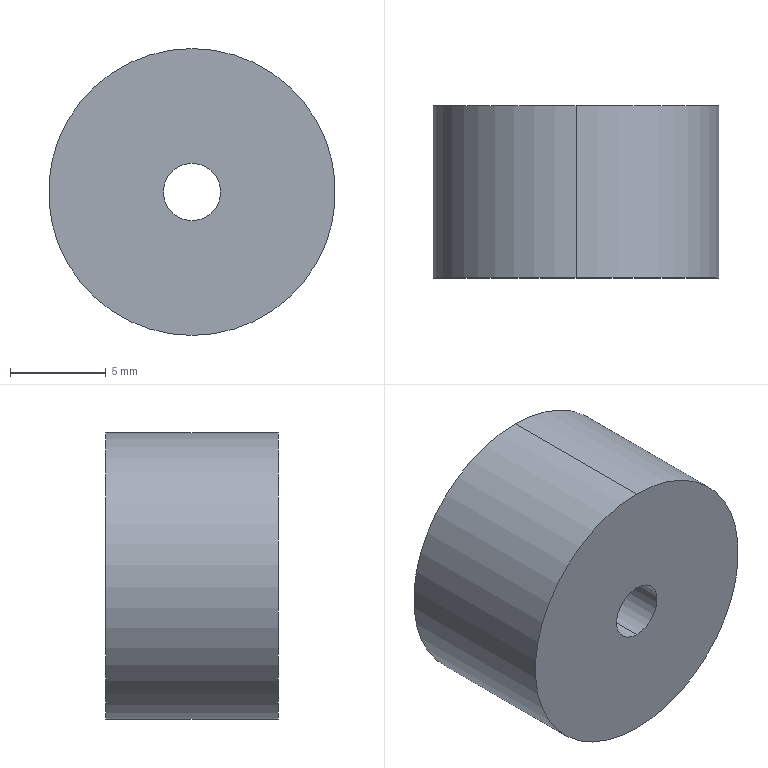Part | STEP file | SM140A-20-1140D-140A-600 Buffer pad | 1 solid | 9 faces | box 15 x 9 x 15 mm | volume 1428 mm3 | cylinder 6 | plane 3 | commonest cylinder face diameters 3 x2 5.6 x2 15 x2
STEP:
#1=CARTESIAN_POINT('',(0.,0.,0.));
#2=DIRECTION('',(0.,0.,1.));
#3=DIRECTION('',(1.,0.,0.));
#4=AXIS2_PLACEMENT_3D('',#1,#2,#3);
#5=CARTESIAN_POINT('',(0.,3.4,2.8));
#6=VERTEX_POINT('',#5);
#7=CARTESIAN_POINT('',(0.,9.,2.8));
#8=VERTEX_POINT('',#7);
#9=CARTESIAN_POINT('',(0.,3.4,2.8));
#10=DIRECTION('',(0.,1.,0.));
#11=VECTOR('',#10,1.);
#12=LINE('',#9,#11);
#13=CARTESIAN_POINT('',(0.,3.4,0.));
#14=DIRECTION('',(0.,1.,0.));
#15=DIRECTION('',(0.,0.,1.));
#16=AXIS2_PLACEMENT_3D('',#13,#14,#15);
#17=CYLINDRICAL_SURFACE('',#16,2.8);
#18=CARTESIAN_POINT('',(6.283,0.));
#19=DIRECTION('',(0.,1.));
#20=VECTOR('',#19,1.);
#21=LINE('',#18,#20);
#22=(GEOMETRIC_REPRESENTATION_CONTEXT(2)PARAMETRIC_REPRESENTATION_CONTEXT()REPRESENTATION_CONTEXT('',''));
#23=DEFINITIONAL_REPRESENTATION('',(#21),#22);
#24=PCURVE('',#17,#23);
#25=CARTESIAN_POINT('',(0.,3.4,0.));
#26=DIRECTION('',(0.,1.,0.));
#27=DIRECTION('',(0.,0.,1.));
#28=AXIS2_PLACEMENT_3D('',#25,#26,#27);
#29=CYLINDRICAL_SURFACE('',#28,2.8);
#30=CARTESIAN_POINT('',(0.,0.));
#31=DIRECTION('',(0.,1.));
#32=VECTOR('',#31,1.);
#33=LINE('',#30,#32);
#34=(GEOMETRIC_REPRESENTATION_CONTEXT(2)PARAMETRIC_REPRESENTATION_CONTEXT()REPRESENTATION_CONTEXT('',''));
#35=DEFINITIONAL_REPRESENTATION('',(#33),#34);
#36=PCURVE('',#29,#35);
#37=SURFACE_CURVE('',#12,(#24,#36),.PCURVE_S1.);
#38=EDGE_CURVE('',#6,#8,#37,.T.);
#39=ORIENTED_EDGE('',*,*,#38,.T.);
#40=CARTESIAN_POINT('',(0.,9.,-2.8));
#41=VERTEX_POINT('',#40);
#42=CARTESIAN_POINT('',(0.,9.,0.));
#43=DIRECTION('',(0.,1.,0.));
#44=DIRECTION('',(0.,0.,1.));
#45=AXIS2_PLACEMENT_3D('',#42,#43,#44);
#46=CIRCLE('',#45,2.8);
#47=CARTESIAN_POINT('',(0.,5.6));
#48=DIRECTION('',(1.,0.));
#49=VECTOR('',#48,1.);
#50=LINE('',#47,#49);
#51=(GEOMETRIC_REPRESENTATION_CONTEXT(2)PARAMETRIC_REPRESENTATION_CONTEXT()REPRESENTATION_CONTEXT('',''));
#52=DEFINITIONAL_REPRESENTATION('',(#50),#51);
#53=PCURVE('',#17,#52);
#54=CARTESIAN_POINT('',(0.,9.,0.));
#55=DIRECTION('',(0.,1.,0.));
#56=DIRECTION('',(0.,0.,1.));
#57=AXIS2_PLACEMENT_3D('',#54,#55,#56);
#58=PLANE('',#57);
#59=CARTESIAN_POINT('',(0.,0.));
#60=DIRECTION('',(1.,0.));
#61=AXIS2_PLACEMENT_2D('',#59,#60);
#62=CIRCLE('',#61,2.8);
#63=(GEOMETRIC_REPRESENTATION_CONTEXT(2)PARAMETRIC_REPRESENTATION_CONTEXT()REPRESENTATION_CONTEXT('',''));
#64=DEFINITIONAL_REPRESENTATION('',(#62),#63);
#65=PCURVE('',#58,#64);
#66=SURFACE_CURVE('',#46,(#53,#65),.PCURVE_S1.);
#67=EDGE_CURVE('',#41,#8,#66,.T.);
#68=ORIENTED_EDGE('',*,*,#67,.F.);
#69=CARTESIAN_POINT('',(0.,3.4,-2.8));
#70=VERTEX_POINT('',#69);
#71=CARTESIAN_POINT('',(0.,3.4,-2.8));
#72=DIRECTION('',(0.,1.,0.));
#73=VECTOR('',#72,1.);
#74=LINE('',#71,#73);
#75=CARTESIAN_POINT('',(3.142,0.));
#76=DIRECTION('',(0.,1.));
#77=VECTOR('',#76,1.);
#78=LINE('',#75,#77);
#79=(GEOMETRIC_REPRESENTATION_CONTEXT(2)PARAMETRIC_REPRESENTATION_CONTEXT()REPRESENTATION_CONTEXT('',''));
#80=DEFINITIONAL_REPRESENTATION('',(#78),#79);
#81=PCURVE('',#17,#80);
#82=CARTESIAN_POINT('',(3.142,0.));
#83=DIRECTION('',(0.,1.));
#84=VECTOR('',#83,1.);
#85=LINE('',#82,#84);
#86=(GEOMETRIC_REPRESENTATION_CONTEXT(2)PARAMETRIC_REPRESENTATION_CONTEXT()REPRESENTATION_CONTEXT('',''));
#87=DEFINITIONAL_REPRESENTATION('',(#85),#86);
#88=PCURVE('',#29,#87);
#89=SURFACE_CURVE('',#74,(#81,#88),.PCURVE_S1.);
#90=EDGE_CURVE('',#70,#41,#89,.T.);
#91=ORIENTED_EDGE('',*,*,#90,.F.);
#92=CARTESIAN_POINT('',(0.,3.4,0.));
#93=DIRECTION('',(0.,1.,0.));
#94=DIRECTION('',(0.,0.,1.));
#95=AXIS2_PLACEMENT_3D('',#92,#93,#94);
#96=CIRCLE('',#95,2.8);
#97=CARTESIAN_POINT('',(0.,0.));
#98=DIRECTION('',(1.,0.));
#99=VECTOR('',#98,1.);
#100=LINE('',#97,#99);
#101=(GEOMETRIC_REPRESENTATION_CONTEXT(2)PARAMETRIC_REPRESENTATION_CONTEXT()REPRESENTATION_CONTEXT('',''));
#102=DEFINITIONAL_REPRESENTATION('',(#100),#101);
#103=PCURVE('',#17,#102);
#104=CARTESIAN_POINT('',(0.,3.4,0.));
#105=DIRECTION('',(0.,1.,0.));
#106=DIRECTION('',(0.,0.,1.));
#107=AXIS2_PLACEMENT_3D('',#104,#105,#106);
#108=PLANE('',#107);
#109=CARTESIAN_POINT('',(0.,0.));
#110=DIRECTION('',(1.,0.));
#111=AXIS2_PLACEMENT_2D('',#109,#110);
#112=CIRCLE('',#111,2.8);
#113=(GEOMETRIC_REPRESENTATION_CONTEXT(2)PARAMETRIC_REPRESENTATION_CONTEXT()REPRESENTATION_CONTEXT('',''));
#114=DEFINITIONAL_REPRESENTATION('',(#112),#113);
#115=PCURVE('',#108,#114);
#116=SURFACE_CURVE('',#96,(#103,#115),.PCURVE_S1.);
#117=EDGE_CURVE('',#70,#6,#116,.T.);
#118=ORIENTED_EDGE('',*,*,#117,.T.);
#119=EDGE_LOOP('',(#39,#68,#91,#118));
#120=FACE_BOUND('',#119,.F.);
#121=ADVANCED_FACE('',(#120),#17,.F.);
#122=CARTESIAN_POINT('',(0.,9.,7.5));
#123=VERTEX_POINT('',#122);
#124=CARTESIAN_POINT('',(0.,9.,-7.5));
#125=VERTEX_POINT('',#124);
#126=CARTESIAN_POINT('',(0.,9.,0.));
#127=DIRECTION('',(0.,1.,0.));
#128=DIRECTION('',(0.,0.,1.));
#129=AXIS2_PLACEMENT_3D('',#126,#127,#128);
#130=CIRCLE('',#129,7.5);
#131=CARTESIAN_POINT('',(0.,9.,0.));
#132=DIRECTION('',(0.,-1.,0.));
#133=DIRECTION('',(0.,0.,-1.));
#134=AXIS2_PLACEMENT_3D('',#131,#132,#133);
#135=CYLINDRICAL_SURFACE('',#134,7.5);
#136=CARTESIAN_POINT('',(3.142,0.));
#137=DIRECTION('',(-1.,0.));
#138=VECTOR('',#137,1.);
#139=LINE('',#136,#138);
#140=(GEOMETRIC_REPRESENTATION_CONTEXT(2)PARAMETRIC_REPRESENTATION_CONTEXT()REPRESENTATION_CONTEXT('',''));
#141=DEFINITIONAL_REPRESENTATION('',(#139),#140);
#142=PCURVE('',#135,#141);
#143=CARTESIAN_POINT('',(0.,0.));
#144=DIRECTION('',(1.,0.));
#145=AXIS2_PLACEMENT_2D('',#143,#144);
#146=CIRCLE('',#145,7.5);
#147=(GEOMETRIC_REPRESENTATION_CONTEXT(2)PARAMETRIC_REPRESENTATION_CONTEXT()REPRESENTATION_CONTEXT('',''));
#148=DEFINITIONAL_REPRESENTATION('',(#146),#147);
#149=PCURVE('',#58,#148);
#150=SURFACE_CURVE('',#130,(#142,#149),.PCURVE_S1.);
#151=EDGE_CURVE('',#123,#125,#150,.T.);
#152=ORIENTED_EDGE('',*,*,#151,.F.);
#153=CARTESIAN_POINT('',(0.,0.,7.5));
#154=VERTEX_POINT('',#153);
#155=CARTESIAN_POINT('',(0.,9.,7.5));
#156=DIRECTION('',(0.,-1.,0.));
#157=VECTOR('',#156,1.);
#158=LINE('',#155,#157);
#159=CARTESIAN_POINT('',(3.142,0.));
#160=DIRECTION('',(0.,1.));
#161=VECTOR('',#160,1.);
#162=LINE('',#159,#161);
#163=(GEOMETRIC_REPRESENTATION_CONTEXT(2)PARAMETRIC_REPRESENTATION_CONTEXT()REPRESENTATION_CONTEXT('',''));
#164=DEFINITIONAL_REPRESENTATION('',(#162),#163);
#165=PCURVE('',#135,#164);
#166=CARTESIAN_POINT('',(0.,9.,0.));
#167=DIRECTION('',(0.,-1.,0.));
#168=DIRECTION('',(0.,0.,-1.));
#169=AXIS2_PLACEMENT_3D('',#166,#167,#168);
#170=CYLINDRICAL_SURFACE('',#169,7.5);
#171=CARTESIAN_POINT('',(3.142,0.));
#172=DIRECTION('',(0.,1.));
#173=VECTOR('',#172,1.);
#174=LINE('',#171,#173);
#175=(GEOMETRIC_REPRESENTATION_CONTEXT(2)PARAMETRIC_REPRESENTATION_CONTEXT()REPRESENTATION_CONTEXT('',''));
#176=DEFINITIONAL_REPRESENTATION('',(#174),#175);
#177=PCURVE('',#170,#176);
#178=SURFACE_CURVE('',#158,(#165,#177),.PCURVE_S1.);
#179=EDGE_CURVE('',#123,#154,#178,.T.);
#180=ORIENTED_EDGE('',*,*,#179,.T.);
#181=CARTESIAN_POINT('',(0.,0.,-7.5));
#182=VERTEX_POINT('',#181);
#183=CARTESIAN_POINT('',(0.,0.,0.));
#184=DIRECTION('',(0.,1.,0.));
#185=DIRECTION('',(0.,0.,1.));
#186=AXIS2_PLACEMENT_3D('',#183,#184,#185);
#187=CIRCLE('',#186,7.5);
#188=CARTESIAN_POINT('',(3.142,9.));
#189=DIRECTION('',(-1.,0.));
#190=VECTOR('',#189,1.);
#191=LINE('',#188,#190);
#192=(GEOMETRIC_REPRESENTATION_CONTEXT(2)PARAMETRIC_REPRESENTATION_CONTEXT()REPRESENTATION_CONTEXT('',''));
#193=DEFINITIONAL_REPRESENTATION('',(#191),#192);
#194=PCURVE('',#135,#193);
#195=CARTESIAN_POINT('',(0.,0.,0.));
#196=DIRECTION('',(0.,1.,0.));
#197=DIRECTION('',(0.,0.,1.));
#198=AXIS2_PLACEMENT_3D('',#195,#196,#197);
#199=PLANE('',#198);
#200=CARTESIAN_POINT('',(0.,0.));
#201=DIRECTION('',(1.,0.));
#202=AXIS2_PLACEMENT_2D('',#200,#201);
#203=CIRCLE('',#202,7.5);
#204=(GEOMETRIC_REPRESENTATION_CONTEXT(2)PARAMETRIC_REPRESENTATION_CONTEXT()REPRESENTATION_CONTEXT('',''));
#205=DEFINITIONAL_REPRESENTATION('',(#203),#204);
#206=PCURVE('',#199,#205);
#207=SURFACE_CURVE('',#187,(#194,#206),.PCURVE_S1.);
#208=EDGE_CURVE('',#154,#182,#207,.T.);
#209=ORIENTED_EDGE('',*,*,#208,.T.);
#210=CARTESIAN_POINT('',(0.,9.,-7.5));
#211=DIRECTION('',(0.,-1.,0.));
#212=VECTOR('',#211,1.);
#213=LINE('',#210,#212);
#214=CARTESIAN_POINT('',(0.,0.));
#215=DIRECTION('',(0.,1.));
#216=VECTOR('',#215,1.);
#217=LINE('',#214,#216);
#218=(GEOMETRIC_REPRESENTATION_CONTEXT(2)PARAMETRIC_REPRESENTATION_CONTEXT()REPRESENTATION_CONTEXT('',''));
#219=DEFINITIONAL_REPRESENTATION('',(#217),#218);
#220=PCURVE('',#135,#219);
#221=CARTESIAN_POINT('',(6.283,0.));
#222=DIRECTION('',(0.,1.));
#223=VECTOR('',#222,1.);
#224=LINE('',#221,#223);
#225=(GEOMETRIC_REPRESENTATION_CONTEXT(2)PARAMETRIC_REPRESENTATION_CONTEXT()REPRESENTATION_CONTEXT('',''));
#226=DEFINITIONAL_REPRESENTATION('',(#224),#225);
#227=PCURVE('',#170,#226);
#228=SURFACE_CURVE('',#213,(#220,#227),.PCURVE_S1.);
#229=EDGE_CURVE('',#125,#182,#228,.T.);
#230=ORIENTED_EDGE('',*,*,#229,.F.);
#231=EDGE_LOOP('',(#152,#180,#209,#230));
#232=FACE_BOUND('',#231,.T.);
#233=ADVANCED_FACE('',(#232),#135,.T.);
#234=CARTESIAN_POINT('',(0.,0.,1.5));
#235=VERTEX_POINT('',#234);
#236=CARTESIAN_POINT('',(0.,3.4,1.5));
#237=VERTEX_POINT('',#236);
#238=CARTESIAN_POINT('',(0.,0.,1.5));
#239=DIRECTION('',(0.,1.,0.));
#240=VECTOR('',#239,1.);
#241=LINE('',#238,#240);
#242=CARTESIAN_POINT('',(0.,0.,0.));
#243=DIRECTION('',(0.,1.,0.));
#244=DIRECTION('',(0.,0.,1.));
#245=AXIS2_PLACEMENT_3D('',#242,#243,#244);
#246=CYLINDRICAL_SURFACE('',#245,1.5);
#247=CARTESIAN_POINT('',(6.283,0.));
#248=DIRECTION('',(0.,1.));
#249=VECTOR('',#248,1.);
#250=LINE('',#247,#249);
#251=(GEOMETRIC_REPRESENTATION_CONTEXT(2)PARAMETRIC_REPRESENTATION_CONTEXT()REPRESENTATION_CONTEXT('',''));
#252=DEFINITIONAL_REPRESENTATION('',(#250),#251);
#253=PCURVE('',#246,#252);
#254=CARTESIAN_POINT('',(0.,0.,0.));
#255=DIRECTION('',(0.,1.,0.));
#256=DIRECTION('',(0.,0.,1.));
#257=AXIS2_PLACEMENT_3D('',#254,#255,#256);
#258=CYLINDRICAL_SURFACE('',#257,1.5);
#259=CARTESIAN_POINT('',(0.,0.));
#260=DIRECTION('',(0.,1.));
#261=VECTOR('',#260,1.);
#262=LINE('',#259,#261);
#263=(GEOMETRIC_REPRESENTATION_CONTEXT(2)PARAMETRIC_REPRESENTATION_CONTEXT()REPRESENTATION_CONTEXT('',''));
#264=DEFINITIONAL_REPRESENTATION('',(#262),#263);
#265=PCURVE('',#258,#264);
#266=SURFACE_CURVE('',#241,(#253,#265),.PCURVE_S1.);
#267=EDGE_CURVE('',#235,#237,#266,.T.);
#268=ORIENTED_EDGE('',*,*,#267,.T.);
#269=CARTESIAN_POINT('',(0.,3.4,-1.5));
#270=VERTEX_POINT('',#269);
#271=CARTESIAN_POINT('',(0.,3.4,0.));
#272=DIRECTION('',(0.,-1.,0.));
#273=DIRECTION('',(0.,0.,1.));
#274=AXIS2_PLACEMENT_3D('',#271,#272,#273);
#275=CIRCLE('',#274,1.5);
#276=CARTESIAN_POINT('',(6.283,3.4));
#277=DIRECTION('',(-1.,0.));
#278=VECTOR('',#277,1.);
#279=LINE('',#276,#278);
#280=(GEOMETRIC_REPRESENTATION_CONTEXT(2)PARAMETRIC_REPRESENTATION_CONTEXT()REPRESENTATION_CONTEXT('',''));
#281=DEFINITIONAL_REPRESENTATION('',(#279),#280);
#282=PCURVE('',#246,#281);
#283=CARTESIAN_POINT('',(1.5,0.));
#284=CARTESIAN_POINT('',(1.5,-2.598));
#285=CARTESIAN_POINT('',(-0.75,-1.299));
#286=CARTESIAN_POINT('',(-3.,0.));
#287=CARTESIAN_POINT('',(-0.75,1.299));
#288=CARTESIAN_POINT('',(1.5,2.598));
#289=CARTESIAN_POINT('',(1.5,0.));
#290=(BOUNDED_CURVE()B_SPLINE_CURVE(2,(#283,#284,#285,#286,#287,#288,#289),.UNSPECIFIED.,.T.,.F.)B_SPLINE_CURVE_WITH_KNOTS((1,2,2,2,2,1),(-2.094,0.,2.094,4.189,6.283,8.378),.UNSPECIFIED.)CURVE()GEOMETRIC_REPRESENTATION_ITEM()RATIONAL_B_SPLINE_CURVE((1.,0.5,1.,0.5,1.,0.5,1.))REPRESENTATION_ITEM(''));
#291=(GEOMETRIC_REPRESENTATION_CONTEXT(2)PARAMETRIC_REPRESENTATION_CONTEXT()REPRESENTATION_CONTEXT('',''));
#292=DEFINITIONAL_REPRESENTATION('',(#290),#291);
#293=PCURVE('',#108,#292);
#294=SURFACE_CURVE('',#275,(#282,#293),.PCURVE_S1.);
#295=EDGE_CURVE('',#237,#270,#294,.T.);
#296=ORIENTED_EDGE('',*,*,#295,.T.);
#297=CARTESIAN_POINT('',(0.,0.,-1.5));
#298=VERTEX_POINT('',#297);
#299=CARTESIAN_POINT('',(0.,0.,-1.5));
#300=DIRECTION('',(0.,1.,0.));
#301=VECTOR('',#300,1.);
#302=LINE('',#299,#301);
#303=CARTESIAN_POINT('',(3.142,0.));
#304=DIRECTION('',(0.,1.));
#305=VECTOR('',#304,1.);
#306=LINE('',#303,#305);
#307=(GEOMETRIC_REPRESENTATION_CONTEXT(2)PARAMETRIC_REPRESENTATION_CONTEXT()REPRESENTATION_CONTEXT('',''));
#308=DEFINITIONAL_REPRESENTATION('',(#306),#307);
#309=PCURVE('',#246,#308);
#310=CARTESIAN_POINT('',(3.142,0.));
#311=DIRECTION('',(0.,1.));
#312=VECTOR('',#311,1.);
#313=LINE('',#310,#312);
#314=(GEOMETRIC_REPRESENTATION_CONTEXT(2)PARAMETRIC_REPRESENTATION_CONTEXT()REPRESENTATION_CONTEXT('',''));
#315=DEFINITIONAL_REPRESENTATION('',(#313),#314);
#316=PCURVE('',#258,#315);
#317=SURFACE_CURVE('',#302,(#309,#316),.PCURVE_S1.);
#318=EDGE_CURVE('',#298,#270,#317,.T.);
#319=ORIENTED_EDGE('',*,*,#318,.F.);
#320=CARTESIAN_POINT('',(0.,0.,0.));
#321=DIRECTION('',(0.,1.,0.));
#322=DIRECTION('',(0.,0.,1.));
#323=AXIS2_PLACEMENT_3D('',#320,#321,#322);
#324=CIRCLE('',#323,1.5);
#325=CARTESIAN_POINT('',(0.,0.));
#326=DIRECTION('',(1.,0.));
#327=VECTOR('',#326,1.);
#328=LINE('',#325,#327);
#329=(GEOMETRIC_REPRESENTATION_CONTEXT(2)PARAMETRIC_REPRESENTATION_CONTEXT()REPRESENTATION_CONTEXT('',''));
#330=DEFINITIONAL_REPRESENTATION('',(#328),#329);
#331=PCURVE('',#246,#330);
#332=CARTESIAN_POINT('',(0.,0.));
#333=DIRECTION('',(1.,0.));
#334=AXIS2_PLACEMENT_2D('',#332,#333);
#335=CIRCLE('',#334,1.5);
#336=(GEOMETRIC_REPRESENTATION_CONTEXT(2)PARAMETRIC_REPRESENTATION_CONTEXT()REPRESENTATION_CONTEXT('',''));
#337=DEFINITIONAL_REPRESENTATION('',(#335),#336);
#338=PCURVE('',#199,#337);
#339=SURFACE_CURVE('',#324,(#331,#338),.PCURVE_S1.);
#340=EDGE_CURVE('',#298,#235,#339,.T.);
#341=ORIENTED_EDGE('',*,*,#340,.T.);
#342=EDGE_LOOP('',(#268,#296,#319,#341));
#343=FACE_BOUND('',#342,.F.);
#344=ADVANCED_FACE('',(#343),#246,.F.);
#345=CARTESIAN_POINT('',(0.,3.4,0.));
#346=DIRECTION('',(0.,-1.,0.));
#347=DIRECTION('',(0.,0.,1.));
#348=AXIS2_PLACEMENT_3D('',#345,#346,#347);
#349=CIRCLE('',#348,1.5);
#350=CARTESIAN_POINT('',(6.283,3.4));
#351=DIRECTION('',(-1.,0.));
#352=VECTOR('',#351,1.);
#353=LINE('',#350,#352);
#354=(GEOMETRIC_REPRESENTATION_CONTEXT(2)PARAMETRIC_REPRESENTATION_CONTEXT()REPRESENTATION_CONTEXT('',''));
#355=DEFINITIONAL_REPRESENTATION('',(#353),#354);
#356=PCURVE('',#258,#355);
#357=CARTESIAN_POINT('',(1.5,0.));
#358=CARTESIAN_POINT('',(1.5,-2.598));
#359=CARTESIAN_POINT('',(-0.75,-1.299));
#360=CARTESIAN_POINT('',(-3.,0.));
#361=CARTESIAN_POINT('',(-0.75,1.299));
#362=CARTESIAN_POINT('',(1.5,2.598));
#363=CARTESIAN_POINT('',(1.5,0.));
#364=(BOUNDED_CURVE()B_SPLINE_CURVE(2,(#357,#358,#359,#360,#361,#362,#363),.UNSPECIFIED.,.T.,.F.)B_SPLINE_CURVE_WITH_KNOTS((1,2,2,2,2,1),(-2.094,0.,2.094,4.189,6.283,8.378),.UNSPECIFIED.)CURVE()GEOMETRIC_REPRESENTATION_ITEM()RATIONAL_B_SPLINE_CURVE((1.,0.5,1.,0.5,1.,0.5,1.))REPRESENTATION_ITEM(''));
#365=(GEOMETRIC_REPRESENTATION_CONTEXT(2)PARAMETRIC_REPRESENTATION_CONTEXT()REPRESENTATION_CONTEXT('',''));
#366=DEFINITIONAL_REPRESENTATION('',(#364),#365);
#367=PCURVE('',#108,#366);
#368=SURFACE_CURVE('',#349,(#356,#367),.PCURVE_S1.);
#369=EDGE_CURVE('',#270,#237,#368,.T.);
#370=ORIENTED_EDGE('',*,*,#369,.T.);
#371=ORIENTED_EDGE('',*,*,#267,.F.);
#372=CARTESIAN_POINT('',(0.,0.,0.));
#373=DIRECTION('',(0.,1.,0.));
#374=DIRECTION('',(0.,0.,1.));
#375=AXIS2_PLACEMENT_3D('',#372,#373,#374);
#376=CIRCLE('',#375,1.5);
#377=CARTESIAN_POINT('',(0.,0.));
#378=DIRECTION('',(1.,0.));
#379=VECTOR('',#378,1.);
#380=LINE('',#377,#379);
#381=(GEOMETRIC_REPRESENTATION_CONTEXT(2)PARAMETRIC_REPRESENTATION_CONTEXT()REPRESENTATION_CONTEXT('',''));
#382=DEFINITIONAL_REPRESENTATION('',(#380),#381);
#383=PCURVE('',#258,#382);
#384=CARTESIAN_POINT('',(0.,0.));
#385=DIRECTION('',(1.,0.));
#386=AXIS2_PLACEMENT_2D('',#384,#385);
#387=CIRCLE('',#386,1.5);
#388=(GEOMETRIC_REPRESENTATION_CONTEXT(2)PARAMETRIC_REPRESENTATION_CONTEXT()REPRESENTATION_CONTEXT('',''));
#389=DEFINITIONAL_REPRESENTATION('',(#387),#388);
#390=PCURVE('',#199,#389);
#391=SURFACE_CURVE('',#376,(#383,#390),.PCURVE_S1.);
#392=EDGE_CURVE('',#235,#298,#391,.T.);
#393=ORIENTED_EDGE('',*,*,#392,.T.);
#394=ORIENTED_EDGE('',*,*,#318,.T.);
#395=EDGE_LOOP('',(#370,#371,#393,#394));
#396=FACE_BOUND('',#395,.F.);
#397=ADVANCED_FACE('',(#396),#258,.F.);
#398=ORIENTED_EDGE('',*,*,#179,.F.);
#399=CARTESIAN_POINT('',(0.,9.,0.));
#400=DIRECTION('',(0.,1.,0.));
#401=DIRECTION('',(0.,0.,1.));
#402=AXIS2_PLACEMENT_3D('',#399,#400,#401);
#403=CIRCLE('',#402,7.5);
#404=CARTESIAN_POINT('',(9.425,0.));
#405=DIRECTION('',(-1.,0.));
#406=VECTOR('',#405,1.);
#407=LINE('',#404,#406);
#408=(GEOMETRIC_REPRESENTATION_CONTEXT(2)PARAMETRIC_REPRESENTATION_CONTEXT()REPRESENTATION_CONTEXT('',''));
#409=DEFINITIONAL_REPRESENTATION('',(#407),#408);
#410=PCURVE('',#170,#409);
#411=CARTESIAN_POINT('',(0.,0.));
#412=DIRECTION('',(1.,0.));
#413=AXIS2_PLACEMENT_2D('',#411,#412);
#414=CIRCLE('',#413,7.5);
#415=(GEOMETRIC_REPRESENTATION_CONTEXT(2)PARAMETRIC_REPRESENTATION_CONTEXT()REPRESENTATION_CONTEXT('',''));
#416=DEFINITIONAL_REPRESENTATION('',(#414),#415);
#417=PCURVE('',#58,#416);
#418=SURFACE_CURVE('',#403,(#410,#417),.PCURVE_S1.);
#419=EDGE_CURVE('',#125,#123,#418,.T.);
#420=ORIENTED_EDGE('',*,*,#419,.F.);
#421=ORIENTED_EDGE('',*,*,#229,.T.);
#422=CARTESIAN_POINT('',(0.,0.,0.));
#423=DIRECTION('',(0.,1.,0.));
#424=DIRECTION('',(0.,0.,1.));
#425=AXIS2_PLACEMENT_3D('',#422,#423,#424);
#426=CIRCLE('',#425,7.5);
#427=CARTESIAN_POINT('',(9.425,9.));
#428=DIRECTION('',(-1.,0.));
#429=VECTOR('',#428,1.);
#430=LINE('',#427,#429);
#431=(GEOMETRIC_REPRESENTATION_CONTEXT(2)PARAMETRIC_REPRESENTATION_CONTEXT()REPRESENTATION_CONTEXT('',''));
#432=DEFINITIONAL_REPRESENTATION('',(#430),#431);
#433=PCURVE('',#170,#432);
#434=CARTESIAN_POINT('',(0.,0.));
#435=DIRECTION('',(1.,0.));
#436=AXIS2_PLACEMENT_2D('',#434,#435);
#437=CIRCLE('',#436,7.5);
#438=(GEOMETRIC_REPRESENTATION_CONTEXT(2)PARAMETRIC_REPRESENTATION_CONTEXT()REPRESENTATION_CONTEXT('',''));
#439=DEFINITIONAL_REPRESENTATION('',(#437),#438);
#440=PCURVE('',#199,#439);
#441=SURFACE_CURVE('',#426,(#433,#440),.PCURVE_S1.);
#442=EDGE_CURVE('',#182,#154,#441,.T.);
#443=ORIENTED_EDGE('',*,*,#442,.T.);
#444=EDGE_LOOP('',(#398,#420,#421,#443));
#445=FACE_BOUND('',#444,.T.);
#446=ADVANCED_FACE('',(#445),#170,.T.);
#447=CARTESIAN_POINT('',(0.,9.,0.));
#448=DIRECTION('',(0.,1.,0.));
#449=DIRECTION('',(0.,0.,1.));
#450=AXIS2_PLACEMENT_3D('',#447,#448,#449);
#451=CIRCLE('',#450,2.8);
#452=CARTESIAN_POINT('',(0.,0.));
#453=DIRECTION('',(1.,0.));
#454=AXIS2_PLACEMENT_2D('',#452,#453);
#455=CIRCLE('',#454,2.8);
#456=(GEOMETRIC_REPRESENTATION_CONTEXT(2)PARAMETRIC_REPRESENTATION_CONTEXT()REPRESENTATION_CONTEXT('',''));
#457=DEFINITIONAL_REPRESENTATION('',(#455),#456);
#458=PCURVE('',#58,#457);
#459=CARTESIAN_POINT('',(0.,5.6));
#460=DIRECTION('',(1.,0.));
#461=VECTOR('',#460,1.);
#462=LINE('',#459,#461);
#463=(GEOMETRIC_REPRESENTATION_CONTEXT(2)PARAMETRIC_REPRESENTATION_CONTEXT()REPRESENTATION_CONTEXT('',''));
#464=DEFINITIONAL_REPRESENTATION('',(#462),#463);
#465=PCURVE('',#29,#464);
#466=SURFACE_CURVE('',#451,(#458,#465),.PCURVE_S1.);
#467=EDGE_CURVE('',#8,#41,#466,.T.);
#468=ORIENTED_EDGE('',*,*,#467,.F.);
#469=ORIENTED_EDGE('',*,*,#67,.F.);
#470=EDGE_LOOP('',(#468,#469));
#471=FACE_BOUND('',#470,.T.);
#472=ORIENTED_EDGE('',*,*,#419,.T.);
#473=ORIENTED_EDGE('',*,*,#151,.T.);
#474=EDGE_LOOP('',(#472,#473));
#475=FACE_BOUND('',#474,.T.);
#476=ADVANCED_FACE('',(#471,#475),#58,.T.);
#477=ORIENTED_EDGE('',*,*,#392,.T.);
#478=ORIENTED_EDGE('',*,*,#340,.T.);
#479=EDGE_LOOP('',(#477,#478));
#480=FACE_BOUND('',#479,.T.);
#481=ORIENTED_EDGE('',*,*,#442,.F.);
#482=ORIENTED_EDGE('',*,*,#208,.F.);
#483=EDGE_LOOP('',(#481,#482));
#484=FACE_BOUND('',#483,.T.);
#485=ADVANCED_FACE('',(#480,#484),#199,.F.);
#486=CARTESIAN_POINT('',(0.,3.4,0.));
#487=DIRECTION('',(0.,1.,0.));
#488=DIRECTION('',(0.,0.,1.));
#489=AXIS2_PLACEMENT_3D('',#486,#487,#488);
#490=CIRCLE('',#489,2.8);
#491=CARTESIAN_POINT('',(0.,0.));
#492=DIRECTION('',(1.,0.));
#493=AXIS2_PLACEMENT_2D('',#491,#492);
#494=CIRCLE('',#493,2.8);
#495=(GEOMETRIC_REPRESENTATION_CONTEXT(2)PARAMETRIC_REPRESENTATION_CONTEXT()REPRESENTATION_CONTEXT('',''));
#496=DEFINITIONAL_REPRESENTATION('',(#494),#495);
#497=PCURVE('',#108,#496);
#498=CARTESIAN_POINT('',(0.,0.));
#499=DIRECTION('',(1.,0.));
#500=VECTOR('',#499,1.);
#501=LINE('',#498,#500);
#502=(GEOMETRIC_REPRESENTATION_CONTEXT(2)PARAMETRIC_REPRESENTATION_CONTEXT()REPRESENTATION_CONTEXT('',''));
#503=DEFINITIONAL_REPRESENTATION('',(#501),#502);
#504=PCURVE('',#29,#503);
#505=SURFACE_CURVE('',#490,(#497,#504),.PCURVE_S1.);
#506=EDGE_CURVE('',#6,#70,#505,.T.);
#507=ORIENTED_EDGE('',*,*,#506,.T.);
#508=ORIENTED_EDGE('',*,*,#117,.T.);
#509=EDGE_LOOP('',(#507,#508));
#510=FACE_BOUND('',#509,.T.);
#511=ORIENTED_EDGE('',*,*,#295,.T.);
#512=ORIENTED_EDGE('',*,*,#369,.T.);
#513=EDGE_LOOP('',(#511,#512));
#514=FACE_BOUND('',#513,.T.);
#515=ADVANCED_FACE('',(#510,#514),#108,.T.);
#516=ORIENTED_EDGE('',*,*,#467,.F.);
#517=ORIENTED_EDGE('',*,*,#38,.F.);
#518=ORIENTED_EDGE('',*,*,#506,.T.);
#519=ORIENTED_EDGE('',*,*,#90,.T.);
#520=EDGE_LOOP('',(#516,#517,#518,#519));
#521=FACE_BOUND('',#520,.F.);
#522=ADVANCED_FACE('',(#521),#29,.F.);
#523=CLOSED_SHELL('',(#121,#233,#344,#397,#446,#476,#485,#515,#522));
#524=MANIFOLD_SOLID_BREP('',#523);
#525=(LENGTH_UNIT()NAMED_UNIT(*)SI_UNIT(.MILLI.,.METRE.));
#526=UNCERTAINTY_MEASURE_WITH_UNIT(LENGTH_MEASURE(0.0000001),#525,'','');
#527=(NAMED_UNIT(*)PLANE_ANGLE_UNIT()SI_UNIT($,.RADIAN.));
#528=(NAMED_UNIT(*)SI_UNIT($,.STERADIAN.)SOLID_ANGLE_UNIT());
#529=(GEOMETRIC_REPRESENTATION_CONTEXT(3)GLOBAL_UNCERTAINTY_ASSIGNED_CONTEXT((#526))GLOBAL_UNIT_ASSIGNED_CONTEXT((#525,#527,#528))REPRESENTATION_CONTEXT('',''));
#530=ADVANCED_BREP_SHAPE_REPRESENTATION('',(#4,#524),#529);